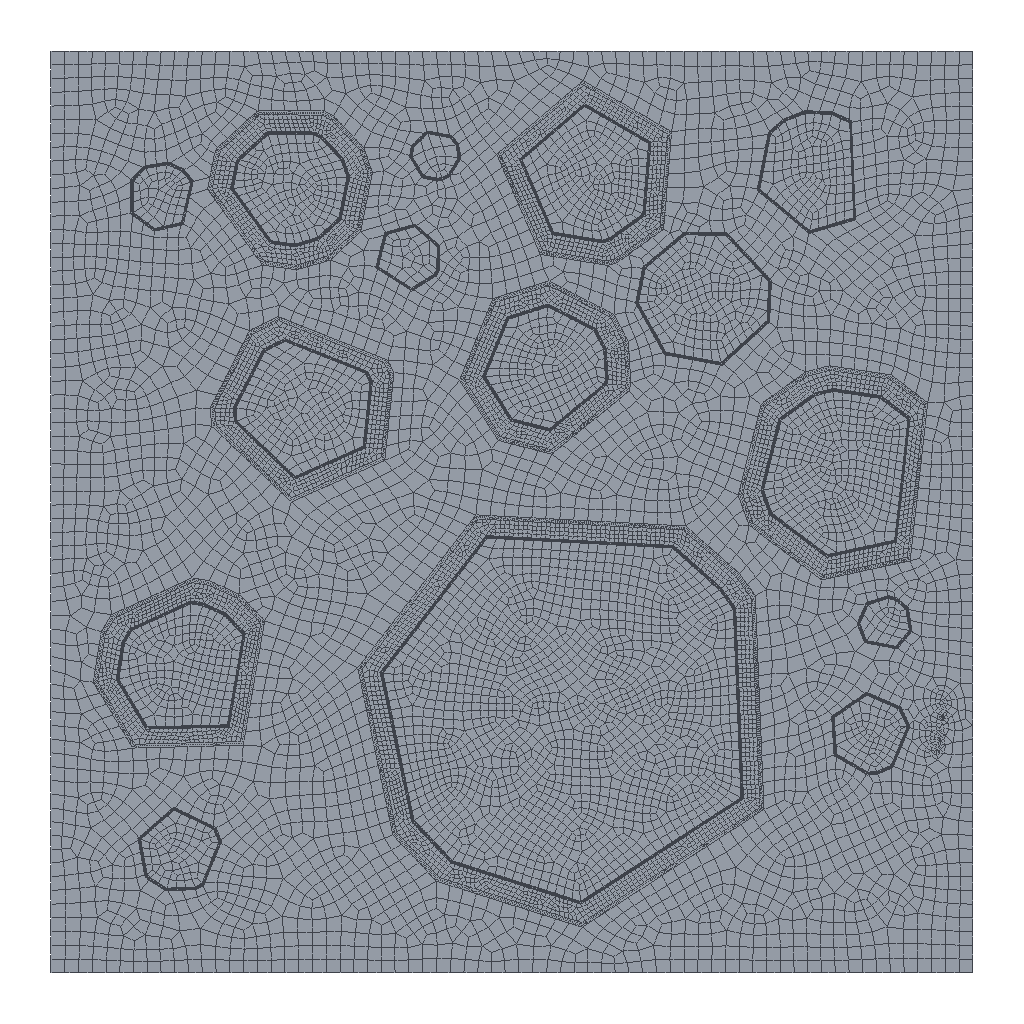Simulation study | abaqus
Set-up summary:
category,name,step,type,value,unit,region
solver,abaqus
solver,version,,,Abaqus/Standard 2020
units,not stated in the deck,,not stated
analysis,deck,,static,static
load_step,Step-1,Step-1,static
load_step,requested,,,1
mesh,nodes,,,46261
mesh,elements,,,36052
element_type,CPS4R,,plane,36052
load,load commands in deck,,count,1
bc,support commands in deck,,count,4
material,GULIAO,,in results
material,JSHANGJIANG,,in results
material,NITZ,,in results
material,NSHAJIANG,,in results
material,OITZ,,in results
check,setup vs results,,match,"per instance, exact: element labels, types and connectivity; labels of the nodes the elements use; coordinates of those nodes at SINGLE_PRECISION in 1 of 5 instance(s)"
Abaqus input file, long lists of numbers shortened:
*Heading
** Job name: Job-1 Model name: model-zaisheng
** Generated by: Abaqus/CAE 2020
*Preprint, echo=NO, model=NO, history=NO, contact=NO
**
** PARTS
**
*Part, name=Part-1
*Node
      1,   77.662,   70.73
      2,   77.846,   75.039
** (3564 more lines like these left out)
*Element, type=CPS4R
  1, 763, 677, 676, 695
  2, 715, 702, 674, 757
** (3245 more lines like these left out)
*Nset, nset=guliao-2, generate
    1,  3566,     1
*Elset, elset=guliao-2, generate
    1,  3247,     1
** Section: guliao-2
*Solid Section, elset=guliao-2, material=guliao
,
*End Part
**
*Part, name=Part-2
*Node
      1,   77.846,   75.039
      2,   77.662,   70.73
** (24805 more lines like these left out)
*Element, type=CPS4R
   1, 12276, 12405, 12781, 12812
   2, 12805, 12781, 12405, 12674
** (18677 more lines like these left out)
*Nset, nset=OITZ-2, generate
     1,  24807,      1
*Elset, elset=OITZ-2, generate
     1,  18679,      1
** Section: OITZ-2
*Solid Section, elset=OITZ-2, material=OITZ
,
*End Part
**
*Part, name=Part-3
*Node
      1,   93.19,   60.231
      2,   91.683,   46.706
** (4621 more lines like these left out)
*Element, type=CPS4R
  1,  253, 1795, 1912,  252
  2,  133, 1891, 1889,  132
** (3725 more lines like these left out)
*Nset, nset=Oshajiang-2, generate
    1,  4623,     1
*Elset, elset=Oshajiang-2, generate
    1,  3727,     1
** Section: Oshajiang-2
*Solid Section, elset=Oshajiang-2, material=Jshangjiang
,
*End Part
**
*Part, name=Part-4
*Node
      1,    94.71,   61.531
      2,   92.879,   45.103
** (9188 more lines like these left out)
*Element, type=CPS4R
  1,  529, 5118, 5141,  528
  2, 5152, 5117,  142,  143
** (6687 more lines like these left out)
*Nset, nset=NITZ, generate
    1,  9190,     1
*Elset, elset=NITZ, generate
    1,  6689,     1
** Section: NITZ-2
*Solid Section, elset=NITZ, material=NITZ
,
*End Part
**
*Part, name=Part-5
*Node
      1,   93.619,   48.661
      2,   94.207,    53.939
** (4073 more lines like these left out)
*Element, type=CPS4R
   1,  400, 2014, 2010, 2510
   2, 1384, 1385,  877,    4
** (3708 more lines like these left out)
*Nset, nset=Nshajiang-2, generate
    1,  4075,     1
*Elset, elset=Nshajiang-2, generate
    1,  3710,     1
** Section: Nshajiang-2
*Solid Section, elset=Nshajiang-2, material=Nshajiang
,
*End Part
**
**
** ASSEMBLY
**
*Assembly, name=Assembly
**
*Instance, name=Part-1-1, part=Part-1
*End Instance
**
*Instance, name=Part-2-1, part=Part-2
*End Instance
**
*Instance, name=Part-3-1, part=Part-3
*End Instance
**
*Instance, name=Part-4-1, part=Part-4
*End Instance
**
*Instance, name=Part-5-1, part=Part-5
*End Instance
**
*Node
      1,          50.,         110.,           0.
*Nset, nset=Set-20
 1,
*Nset, nset=Set-21
 1,
*Nset, nset=Set-22
 1,
*Nset, nset=Set-26
 1,
*Nset, nset=Set-31
 1,
*Nset, nset=Set-35, instance=Part-5-1
  254,  255,  256,  257,  258,  259,  260,  261,  262,  263,  264,  265,  266,  267,  268,  269
  270,  271,  272,  273,  274,  275,  276,  277,  278,  279,  280,  281,  282,  283,  284,  285
** (3 more lines like these left out)
*Elset, elset=Set-35, instance=Part-5-1
   28,   29,   31,  189,  596,  598,  608,  609,  618,  620,  628,  629,  635,  636,  637,  638
  646,  647,  648,  650,  801,  806,  809,  813,  815,  816,  817,  818,  819,  820,  821,  822
** (3 more lines like these left out)
*Nset, nset=Set-39
 1,
*Nset, nset=Set-51
 1,
*Nset, nset=Set-52
 1,
*Nset, nset=Set-RP
 1,
*Nset, nset=m_Set-28
 1,
*Nset, nset=m_Set-33
 1,
*Nset, nset=m_Set-34
 1,
*Nset, nset=m_Set-36
 1,
*Nset, nset=m_Set-37
 1,
*Nset, nset=m_Set-38, instance=Part-2-1
     1,     2,     3,     4,     5,     6,     7,     8,     9,    10,    11,    12,    13,    14,    15,    16
    17,    18,    19,    20,    21,    22,    23,    24,    25,    26,    27,    28,    29,    30,    31,    32
** (544 more lines like these left out)
*Elset, elset=m_Set-38, instance=Part-2-1, generate
    1,  6575,     1
*Nset, nset=s_Set-27
 1,
*Nset, nset=s_Set-37, instance=Part-5-1, generate
    1,  4075,     1
*Elset, elset=s_Set-37, instance=Part-5-1, generate
    1,  3710,     1
*Elset, elset=_m_Surf-2_S4, internal, instance=Part-4-1
    1,   16,   26,   50,   67,   72,   74,   85,   86,   91,   92,   96,   97,  113,  126,  130
  153,  155,  165,  201,  217,  232,  239,  255,  258,  272,  289,  301,  312,  344,  346,  348
** (37 more lines like these left out)
*Elset, elset=_m_Surf-2_S2, internal, instance=Part-4-1
    9,   10,   22,   37,   49,   51,   73,   89,   93,   94,   98,   99,  103,  111,  125,  128
  131,  132,  134,  136,  142,  144,  146,  147,  151,  152,  170,  188,  194,  197,  198,  200
** (47 more lines like these left out)
*Elset, elset=_m_Surf-2_S1, internal, instance=Part-4-1
   27,   29,   58,   62,   63,   70,   71,   76,   77,   81,   85,  107,  119,  148,  190,  266
  330,  333,  334,  336,  374,  462,  470,  565,  606,  608,  639,  640,  653,  655,  667,  777
** (33 more lines like these left out)
*Elset, elset=_m_Surf-2_S3, internal, instance=Part-4-1
   30,   31,   32,   41,   66,   68,   75,   78,   84,  105,  124,  125,  150,  178,  184,  196
  216,  262,  321,  337,  339,  342,  371,  412,  415,  440,  456,  460,  461,  472,  473,  489
** (37 more lines like these left out)
*Surface, type=ELEMENT, name=m_Surf-2
_m_Surf-2_S4, S4
_m_Surf-2_S2, S2
_m_Surf-2_S1, S1
_m_Surf-2_S3, S3
*Elset, elset=_m_Surf-7_S4, internal, instance=Part-3-1
    2,    3,    9,   10,   14,   32,   77,   79,   85,   91,   95,   98,  126,  127,  135,  150
  171,  178,  199,  201,  222,  223,  228,  229,  236,  242,  243,  248,  501,  521,  523,  526
** (14 more lines like these left out)
*Elset, elset=_m_Surf-7_S2, internal, instance=Part-3-1
    4,   66,   80,   88,  198,  200,  204,  227,  230,  234,  245,  246,  247,  250,  330,  420
  502,  503,  511,  524,  531,  533,  554,  560,  598,  601,  606,  610,  611,  642,  653,  665
** (12 more lines like these left out)
*Elset, elset=_m_Surf-7_S3, internal, instance=Part-3-1
   12,   25,   28,   40,   51,   68,   69,   70,   71,   72,   73,   78,  104,  105,  106,  112
  115,  117,  120,  134,  205,  210,  211,  213,  216,  237,  249,  318,  421,  426,  458,  460
** (10 more lines like these left out)
*Elset, elset=_m_Surf-7_S1, internal, instance=Part-3-1
   15,   22,   67,  116,  118,  119,  128,  132,  136,  137,  148,  174,  224,  225,  226,  231
  232,  233,  238,  239,  241,  251,  252,  253,  255,  256,  316,  322,  331,  333,  341,  370
** (9 more lines like these left out)
*Surface, type=ELEMENT, name=m_Surf-7
_m_Surf-7_S4, S4
_m_Surf-7_S2, S2
_m_Surf-7_S3, S3
_m_Surf-7_S1, S1
*Elset, elset=_m_Surf-9_S2, internal, instance=Part-1-1
    3,    4,    6,    8,   19,   24,   28,   31,   40,   41,   44,   45,   46,   52,   58,   70
  178,  193,  195,  211,  212,  213,  216,  221,  228,  249,  250,  255,  259,  261,  269,  271
** (10 more lines like these left out)
*Elset, elset=_m_Surf-9_S4, internal, instance=Part-1-1
    5,    7,   12,   13,   14,   15,   18,   21,   26,   29,   30,   32,   33,   42,   43,   54
   55,  188,  192,  199,  214,  215,  217,  218,  220,  235,  264,  265,  268,  272,  274,  294
** (8 more lines like these left out)
*Elset, elset=_m_Surf-9_S3, internal, instance=Part-1-1
    3,   24,   37,   62,   70,   86,  187,  191,  194,  195,  197,  198,  210,  216,  219,  227
  256,  258,  262,  280,  285,  287,  288,  290,  293,  298,  301,  302,  317,  320,  331,  333
** (6 more lines like these left out)
*Elset, elset=_m_Surf-9_S1, internal, instance=Part-1-1
    9,   13,   39,   63,  188,  201,  202,  208,  220,  226,  236,  265,  267,  268,  274,  286
  306,  315,  337,  357,  374,  377,  378,  386,  387,  402,  405,  416,  431,  468,  475,  484
** (7 more lines like these left out)
*Surface, type=ELEMENT, name=m_Surf-9
_m_Surf-9_S2, S2
_m_Surf-9_S4, S4
_m_Surf-9_S3, S3
_m_Surf-9_S1, S1
*Elset, elset=_s_Surf-2_S3, internal, instance=Part-5-1
    2,    7,    9,   20,   22,   23,   47,   50,   55,   62,   63,   65,   86,   94,   98,  102
  103,  120,  131,  154,  157,  237,  258,  260,  261,  320,  327,  328,  330,  363,  367,  369
** (6 more lines like these left out)
*Elset, elset=_s_Surf-2_S1, internal, instance=Part-5-1
    3,   19,   21,   66,  156,  160,  236,  252,  254,  255,  259,  263,  272,  350,  368,  392
  450,  456,  464,  465,  466,  469,  481,  490,  491,  497,  514,  516,  522,  574,  586,  588
** (5 more lines like these left out)
*Elset, elset=_s_Surf-2_S4, internal, instance=Part-5-1
   12,   53,   57,   72,   93,   99,  219,  235,  248,  269,  270,  271,  448,  501,  502,  570
  573,  730,  739,  742,  751,  790,  945,  973, 1059, 1084, 1176, 1223, 1224, 1227, 1296, 1299
** (1 more lines like these left out)
*Elset, elset=_s_Surf-2_S2, internal, instance=Part-5-1
   56,   74,   79,   80,  119,  217,  234,  247,  262,  276,  321,  364,  366,  411,  444,  447
  449,  451,  498,  517,  571,  580,  581,  634,  681,  683,  713,  732,  733,  740,  743,  746
** (3 more lines like these left out)
*Surface, type=ELEMENT, name=s_Surf-2
_s_Surf-2_S3, S3
_s_Surf-2_S1, S1
_s_Surf-2_S4, S4
_s_Surf-2_S2, S2
*Elset, elset=_s_Surf-4_S1, internal, instance=Part-5-1
  178,  180,  323,  325,  332,  334,  342,  343,  344,  345,  429,  472,  479,  870,  871,  874
  875,  877,  878,  880,  881,  884,  888,  892,  896,  897,  900,  903, 1776, 1789, 1837, 1838
** (1 more lines like these left out)
*Elset, elset=_s_Surf-4_S3, internal, instance=Part-5-1
  430,  473,  477,  483,  488,  489,  492,  866,  869,  918, 1451, 1454, 1457, 1462, 1463, 1470
 1471, 1843, 1844, 1932, 1934
*Elset, elset=_s_Surf-4_S4, internal, instance=Part-5-1
  868,  917, 1787
*Elset, elset=_s_Surf-4_S2, internal, instance=Part-5-1
  901,  904,  907,  908,  912, 1922
*Surface, type=ELEMENT, name=s_Surf-4
_s_Surf-4_S1, S1
_s_Surf-4_S3, S3
_s_Surf-4_S4, S4
_s_Surf-4_S2, S2
*Elset, elset=_s_Surf-5_S1, internal, instance=Part-5-1
  178,  180,  323,  325,  332,  334,  342,  343,  344,  345,  429,  472,  479,  870,  871,  874
  875,  877,  878,  880,  881,  884,  888,  892,  896,  897,  900,  903, 1776, 1789, 1837, 1838
** (1 more lines like these left out)
*Elset, elset=_s_Surf-5_S3, internal, instance=Part-5-1
  430,  473,  477,  483,  488,  489,  492,  866,  869,  918, 1451, 1454, 1457, 1462, 1463, 1470
 1471, 1843, 1844, 1932, 1934
*Elset, elset=_s_Surf-5_S4, internal, instance=Part-5-1
  868,  917, 1787
*Elset, elset=_s_Surf-5_S2, internal, instance=Part-5-1
  901,  904,  907,  908,  912, 1922
*Surface, type=ELEMENT, name=s_Surf-5
_s_Surf-5_S1, S1
_s_Surf-5_S3, S3
_s_Surf-5_S4, S4
_s_Surf-5_S2, S2
*Elset, elset=_s_Surf-6_S4, internal, instance=Part-3-1
    1,   45,   57,   63,   65,   90,   93,   97,  139,  141,  144,  151,  152,  158,  162,  167
  173,  182,  187,  195,  218,  221,  265,  268,  272,  278,  279,  286,  289,  292,  294,  297
** (16 more lines like these left out)
*Elset, elset=_s_Surf-6_S2, internal, instance=Part-3-1
    7,   47,   59,   60,   82,   83,   87,   99,  100,  101,  102,  107,  108,  109,  121,  124
  143,  146,  149,  157,  159,  161,  168,  170,  172,  179,  185,  197,  206,  262,  263,  264
** (18 more lines like these left out)
*Elset, elset=_s_Surf-6_S1, internal, instance=Part-3-1
   13,   24,   27,   31,   34,   36,   42,   49,  110,  131,  141,  152,  164,  188,  257,  274
  281,  290,  313,  349,  390,  391,  505,  509,  517,  518,  525,  530,  564,  569,  570,  584
** (11 more lines like these left out)
*Elset, elset=_s_Surf-6_S3, internal, instance=Part-3-1
   16,   20,   30,   76,  155,  176,  184,  191,  193,  209,  258,  259,  260,  266,  275,  291
  339,  344,  345,  388,  506,  508,  515,  516,  529,  532,  565,  571,  572,  586,  623,  629
** (11 more lines like these left out)
*Surface, type=ELEMENT, name=s_Surf-6
_s_Surf-6_S4, S4
_s_Surf-6_S2, S2
_s_Surf-6_S1, S1
_s_Surf-6_S3, S3
*Elset, elset=_s_Surf-7_S4, internal, instance=Part-2-1
  6579,  6585,  6587,  6588,  6591,  6597,  6598,  6600,  6601,  6606,  6614,  6616,  6620,  6621,  6623,  6625
  6626,  6627,  6628,  6629,  6633,  6637,  6644,  6648,  6649,  6655,  6656,  6658,  6659,  6668,  6669,  6671
** (59 more lines like these left out)
*Elset, elset=_s_Surf-7_S2, internal, instance=Part-2-1
  6583,  6589,  6604,  6605,  6610,  6612,  6618,  6632,  6636,  6639,  6641,  6642,  6650,  6651,  6652,  6673
  6676,  6679,  6680,  6682,  6683,  6688,  6689,  6690,  6699,  6703,  6710,  6784,  6813,  6815,  6823,  6830
** (72 more lines like these left out)
*Elset, elset=_s_Surf-7_S1, internal, instance=Part-2-1
  6691,  6711,  6719,  6727,  6749,  6759,  6760,  6761,  6785,  6806,  6814,  6819,  6822,  6825,  6827,  6831
  6837,  6841,  6851,  6878,  6929,  6930,  6934,  6935,  6997,  7008,  7020,  7060,  7147,  7223,  7243,  7246
** (62 more lines like these left out)
*Elset, elset=_s_Surf-7_S3, internal, instance=Part-2-1
  6715,  6756,  6763,  6767,  6773,  6786,  6790,  6791,  6794,  6797,  6836,  6838,  6840,  6843,  6849,  6854
  6882,  6928,  6983,  6985,  6992,  6993,  6995,  7009,  7017,  7085,  7114,  7149,  7158,  7206,  7217,  7220
** (54 more lines like these left out)
*Surface, type=ELEMENT, name=s_Surf-7
_s_Surf-7_S4, S4
_s_Surf-7_S2, S2
_s_Surf-7_S1, S1
_s_Surf-7_S3, S3
*Elset, elset=_s_Surf-9_S3, internal, instance=Part-2-1
     5,     6,     7,    11,    21,    37,    41,    60,    68,    71,    82,   227,   228,   230,   238,   242
   254,   259,   262,   266,   268,   281,   293,   298,   300,   302,   303,   304,   329,   331,   332,   344
** (94 more lines like these left out)
*Elset, elset=_s_Surf-9_S1, internal, instance=Part-2-1
    12,    18,    19,    22,    27,    29,    31,    39,    47,    48,    57,    59,    64,    65,    67,    75
    78,    80,   120,   235,   239,   246,   269,   271,   276,   280,   289,   290,   296,   299,   308,   327
** (98 more lines like these left out)
*Elset, elset=_s_Surf-9_S2, internal, instance=Part-2-1
    88,    97,   106,   107,   131,   133,   142,   146,   149,   150,   155,   174,   176,   194,   213,   245
   307,   319,   333,   336,   354,   357,   366,   376,   377,   378,   628,   646,   669,   711,   712,   713
** (97 more lines like these left out)
*Elset, elset=_s_Surf-9_S4, internal, instance=Part-2-1
    84,    94,   102,   112,   116,   139,   140,   148,   152,   153,   154,   163,   165,   169,   178,   179
   182,   189,   190,   199,   214,   219,   222,   223,   240,   317,   322,   335,   352,   363,   554,   610
** (80 more lines like these left out)
*Surface, type=ELEMENT, name=s_Surf-9
_s_Surf-9_S3, S3
_s_Surf-9_S1, S1
_s_Surf-9_S2, S2
_s_Surf-9_S4, S4
** Constraint: Constraint-1
*Tie, name=Constraint-1, adjust=yes
m_Surf-2, s_Surf-2
** Constraint: Constraint-2
*Coupling, constraint name=Constraint-2, ref node=m_Set-36, surface=s_Surf-5
*Kinematic
** Constraint: Constraint-3
*Tie, name=Constraint-3, adjust=yes
s_Surf-6, m_Surf-2
** Constraint: Constraint-guliao
*Tie, name=Constraint-guliao, adjust=yes
m_Surf-9, s_Surf-9
** Constraint: Constraint-insert
*Embedded Element, host elset=s_Set-37
m_Set-38
** Constraint: Constraint-p2-p3
*Tie, name=Constraint-p2-p3, adjust=yes
s_Surf-7, m_Surf-7
*End Assembly
*Amplitude, name=Amp-2, definition=SMOOTH STEP
             0.,              0.,           0.001,              1.
*Amplitude, name=Amp-3
             0.,              0.,              1.,              1.
*Amplitude, name=Amp-4, definition=SMOOTH STEP
             0.,              0.,           0.001,              1.
**
** MATERIALS
**
*Material, name=Jshangjiang
*Density
 2.36e-09,
*Elastic
 20396.2, 0.22
*Concrete Damaged Plasticity
36.,    0.1,   1.16,  0.667, 0.0005
*Concrete Compression Hardening
 17.812,          0.
 19.451, 3.76892e-05
 20.955,  7.4105e-05
 22.323, 0.0001172
 23.552, 0.0001671
 24.642, 0.0002238
 25.591, 0.0002874
 26.398,  0.000358
 24.688, 0.000552
 26.246, 0.0005858
 27.373, 0.0006406
  28.038,   0.0007182
  28.251,  0.0008179
 28.058, 0.0009375
 27.529,  0.001074
  26.741,  0.001222
 25.772,  0.00138
 24.688,  0.001543
 23.546,  0.001709
  22.388,  0.001876
 21.244,  0.002043
 20.136,  0.002207
 19.076,  0.002369
 18.072,  0.002529
 17.129,  0.002685
 16.246,  0.002838
 15.422,  0.002989
 14.656,  0.003137
 13.943,  0.003282
 13.281,  0.003424
 12.667,  0.003565
 12.095,  0.003703
 11.564,  0.003839
 9.779,   0.004367
*Concrete Tension Stiffening
 2.06,      0.
 1.92,   2e-05
 1.72,   5e-05
 1.53,   8e-05
 1.37,  0.0001
 1.24, 0.00013
 1.13, 0.00015
 1.04, 0.00017
 0.97, 0.00019
  0.9, 0.00021
 0.85, 0.00024
 0.66, 0.00033
 0.54, 0.00043
 0.47, 0.00052
 0.41, 0.00062
 0.37, 0.00071
 0.34,  0.0008
 0.31, 0.00089
 0.29, 0.00099
*Concrete Compression Damage, tension recovery=1.
        0.,          0.
 0.01172, 3.76892e-05
 0.02118,  7.4105e-05
 0.03113, 0.0001172
  0.04161, 0.0001671
 0.05265, 0.0002238
 0.0643, 0.0002874
 0.07663,  0.000358
   0.1203, 0.000552
  0.1202, 0.0005858
  0.1253, 0.0006406
  0.1355,   0.0007182
  0.1505,  0.0008179
  0.1697, 0.0009375
  0.1927,  0.001074
  0.2186,  0.001222
  0.2468,  0.00138
  0.2767,  0.001543
   0.3076,  0.001709
  0.339,  0.001876
  0.3704,  0.002043
  0.4015,  0.002207
  0.4318,  0.002369
  0.4612,  0.002529
  0.4896,  0.002685
  0.5167,  0.002838
  0.5425,  0.002989
  0.567,  0.003137
  0.5902,  0.003282
   0.612,  0.003424
  0.6326,  0.003565
  0.652,  0.003703
  0.6701,  0.003839
  0.7321,   0.004367
*Concrete Tension Damage
      0.,      0.
 0.1393,   2e-05
 0.2776,   5e-05
 0.3954,   8e-05
 0.4912,  0.0001
 0.5681, 0.00013
 0.6297, 0.00015
 0.6794, 0.00017
 0.7199, 0.00019
 0.7533, 0.00021
 0.781, 0.00024
 0.8675, 0.00033
 0.9105, 0.00043
 0.935, 0.00052
 0.9504, 0.00062
 0.9607, 0.00071
 0.9679,  0.0008
 0.9733, 0.00089
 0.9774, 0.00099
*Material, name=NITZ
*Density
 2.37e-09,
*Elastic
 19263.1, 0.2
*Concrete Damaged Plasticity
30.,    0.1,   1.16,  0.667, 0.0005
*Concrete Compression Hardening
 16.823,          0.
 18.371, 3.76892e-05
  19.791,  7.4105e-05
 21.082, 0.0001172
 22.243, 0.0001671
 23.273, 0.0002238
 24.169, 0.0002874
 24.931,  0.000358
 23.317, 0.000552
 24.788, 0.0005858
 25.852, 0.0006406
 26.48,   0.0007182
 26.681,  0.0008179
 26.499, 0.0009375
 25.999,  0.001074
 25.255,  0.001222
   24.34,  0.00138
 23.317,  0.001543
 22.238,  0.001709
 21.144,  0.001876
 20.064,  0.002043
 19.017,  0.002207
 18.016,  0.002369
 17.068,  0.002529
  16.177,  0.002685
 15.343,  0.002838
 14.565,  0.002989
 13.841,  0.003137
 13.169,  0.003282
 12.544,  0.003424
 11.963,  0.003565
 11.423,  0.003703
 10.922,  0.003839
 9.235,   0.004367
*Concrete Tension Stiffening
 2.06,      0.
 1.92,   2e-05
 1.72,   5e-05
 1.53,   8e-05
 1.37,  0.0001
 1.24, 0.00013
 1.13, 0.00015
 1.04, 0.00017
 0.97, 0.00019
  0.9, 0.00021
 0.85, 0.00024
 0.66, 0.00033
 0.54, 0.00043
 0.47, 0.00052
 0.41, 0.00062
 0.37, 0.00071
 0.34,  0.0008
 0.31, 0.00089
 0.29, 0.00099
*Concrete Compression Damage
        0.,          0.
 0.01172, 3.76892e-05
 0.02118,  7.4105e-05
 0.03113, 0.0001172
  0.04161, 0.0001671
 0.05265, 0.0002238
 0.0643, 0.0002874
 0.07663,  0.000358
   0.1203, 0.000552
  0.1202, 0.0005858
  0.1253, 0.0006406
  0.1355,   0.0007182
  0.1505,  0.0008179
  0.1697, 0.0009375
  0.1927,  0.001074
  0.2186,  0.001222
  0.2468,  0.00138
  0.2767,  0.001543
   0.3076,  0.001709
  0.339,  0.001876
  0.3704,  0.002043
  0.4015,  0.002207
  0.4318,  0.002369
  0.4612,  0.002529
  0.4896,  0.002685
  0.5167,  0.002838
  0.5425,  0.002989
  0.567,  0.003137
  0.5902,  0.003282
   0.612,  0.003424
  0.6326,  0.003565
  0.652,  0.003703
  0.6701,  0.003839
  0.7321,   0.004367
*Concrete Tension Damage
      0.,      0.
 0.1393,   2e-05
 0.2776,   5e-05
 0.3954,   8e-05
 0.4912,  0.0001
 0.5681, 0.00013
 0.6297, 0.00015
 0.6794, 0.00017
 0.7199, 0.00019
 0.7533, 0.00021
 0.781, 0.00024
 0.8675, 0.00033
 0.9105, 0.00043
 0.935, 0.00052
 0.9504, 0.00062
 0.9607, 0.00071
 0.9679,  0.0008
 0.9733, 0.00089
 0.9774, 0.00099
*Material, name=Nshajiang
*Density
 2.38e-09,
*Elastic
 22662.5, 0.22
*Concrete Damaged Plasticity
36.,    0.1,   1.16,  0.667, 0.0005
*Concrete Compression Hardening
 15.14,          0.
 16.534, 3.76892e-05
 17.812,  7.4105e-05
 18.974, 0.0001172
 20.019, 0.0001671
 20.945, 0.0002238
 21.752, 0.0002874
 22.438,  0.000358
 20.985, 0.000552
 22.309, 0.0005858
 23.267, 0.0006406
 23.832,   0.0007182
 24.013,  0.0008179
 23.849, 0.0009375
 23.399,  0.001074
 22.73,  0.001222
  21.906,  0.00138
 20.985,  0.001543
 20.014,  0.001709
 19.03,  0.001876
 18.058,  0.002043
 17.115,  0.002207
 16.214,  0.002369
 15.361,  0.002529
 14.559,  0.002685
 13.809,  0.002838
 13.109,  0.002989
 12.457,  0.003137
 11.852,  0.003282
 11.289,  0.003424
 10.767,  0.003565
  10.281,  0.003703
 9.829,  0.003839
 8.312,   0.004367
*Concrete Tension Stiffening
 2.06,      0.
 1.92,   2e-05
 1.72,   5e-05
 1.53,   8e-05
 1.37,  0.0001
 1.24, 0.00013
 1.13, 0.00015
 1.04, 0.00017
 0.97, 0.00019
  0.9, 0.00021
 0.85, 0.00024
 0.66, 0.00033
 0.54, 0.00043
 0.47, 0.00052
 0.41, 0.00062
 0.37, 0.00071
 0.34,  0.0008
 0.31, 0.00089
 0.29, 0.00099
*Concrete Compression Damage, tension recovery=1.
        0.,          0.
 0.01172, 3.76892e-05
 0.02118,  7.4105e-05
 0.03113, 0.0001172
  0.04161, 0.0001671
 0.05265, 0.0002238
 0.0643, 0.0002874
 0.07663,  0.000358
   0.1203, 0.000552
  0.1202, 0.0005858
  0.1253, 0.0006406
  0.1355,   0.0007182
  0.1505,  0.0008179
  0.1697, 0.0009375
  0.1927,  0.001074
  0.2186,  0.001222
  0.2468,  0.00138
  0.2767,  0.001543
   0.3076,  0.001709
  0.339,  0.001876
  0.3704,  0.002043
  0.4015,  0.002207
  0.4318,  0.002369
  0.4612,  0.002529
  0.4896,  0.002685
  0.5167,  0.002838
  0.5425,  0.002989
  0.567,  0.003137
  0.5902,  0.003282
   0.612,  0.003424
  0.6326,  0.003565
  0.652,  0.003703
  0.6701,  0.003839
  0.7321,   0.004367
*Concrete Tension Damage
      0.,      0.
 0.1393,   2e-05
 0.2776,   5e-05
 0.3954,   8e-05
 0.4912,  0.0001
 0.5681, 0.00013
 0.6297, 0.00015
 0.6794, 0.00017
 0.7199, 0.00019
 0.7533, 0.00021
 0.781, 0.00024
 0.8675, 0.00033
 0.9105, 0.00043
 0.935, 0.00052
 0.9504, 0.00062
 0.9607, 0.00071
 0.9679,  0.0008
 0.9733, 0.00089
 0.9774, 0.00099
*Material, name=OITZ
*Density
 2.37e-09,
*Elastic
 17336.8, 0.2
*Concrete Damaged Plasticity
30.,    0.1,   1.16,  0.667, 0.0005
*Concrete Compression Hardening
 19.791,          0.
 21.613, 3.76892e-05
 23.284,  7.4105e-05
 24.803, 0.0001172
 26.169, 0.0001671
 27.38, 0.0002238
 28.434, 0.0002874
  29.331,  0.000358
 27.432, 0.000552
 29.162, 0.0005858
 30.415, 0.0006406
 31.153,   0.0007182
   31.39,  0.0008179
 31.176, 0.0009375
 30.587,  0.001074
 29.712,  0.001222
 28.635,  0.00138
 27.432,  0.001543
 26.163,  0.001709
 24.876,  0.001876
 23.605,  0.002043
 22.373,  0.002207
 21.195,  0.002369
 20.08,  0.002529
 19.032,  0.002685
 18.051,  0.002838
 17.136,  0.002989
 16.284,  0.003137
 15.493,  0.003282
 14.757,  0.003424
  14.074,  0.003565
 13.439,  0.003703
 12.849,  0.003839
 10.865,   0.004367
*Concrete Tension Stiffening
 2.06,      0.
 1.92,   2e-05
 1.72,   5e-05
 1.53,   8e-05
 1.37,  0.0001
 1.24, 0.00013
 1.13, 0.00015
 1.04, 0.00017
 0.97, 0.00019
  0.9, 0.00021
 0.85, 0.00024
 0.66, 0.00033
 0.54, 0.00043
 0.47, 0.00052
 0.41, 0.00062
 0.37, 0.00071
 0.34,  0.0008
 0.31, 0.00089
 0.29, 0.00099
*Concrete Compression Damage, tension recovery=1.
        0.,          0.
 0.01172, 3.76892e-05
 0.02118,  7.4105e-05
 0.03113, 0.0001172
  0.04161, 0.0001671
 0.05265, 0.0002238
 0.0643, 0.0002874
 0.07663,  0.000358
   0.1203, 0.000552
  0.1202, 0.0005858
  0.1253, 0.0006406
  0.1355,   0.0007182
  0.1505,  0.0008179
  0.1697, 0.0009375
  0.1927,  0.001074
  0.2186,  0.001222
  0.2468,  0.00138
  0.2767,  0.001543
   0.3076,  0.001709
  0.339,  0.001876
  0.3704,  0.002043
  0.4015,  0.002207
  0.4318,  0.002369
  0.4612,  0.002529
  0.4896,  0.002685
  0.5167,  0.002838
  0.5425,  0.002989
  0.567,  0.003137
  0.5902,  0.003282
   0.612,  0.003424
  0.6326,  0.003565
  0.652,  0.003703
  0.6701,  0.003839
  0.7321,   0.004367
*Concrete Tension Damage
      0.,      0.
 0.1393,   2e-05
 0.2776,   5e-05
 0.3954,   8e-05
 0.4912,  0.0001
 0.5681, 0.00013
 0.6297, 0.00015
 0.6794, 0.00017
 0.7199, 0.00019
 0.7533, 0.00021
 0.781, 0.00024
 0.8675, 0.00033
 0.9105, 0.00043
 0.935, 0.00052
 0.9504, 0.00062
 0.9607, 0.00071
 0.9679,  0.0008
 0.9733, 0.00089
 0.9774, 0.00099
*Material, name=guliao
*Density
 2.37e-09,
*Elastic
70000., 0.16
**
** INTERACTION PROPERTIES
**
*Surface Interaction, name=IntProp-1
1.,
*Friction
0.,
*Surface Behavior, pressure-overclosure=HARD
** ----------------------------------------------------------------
**
** STEP: Step-1
**
*Step, name=Step-1, nlgeom=YES, inc=10000
*Static, stabilize=0.0002, allsdtol=0.05, continue=NO
0.001, 1., 1e-09, 1.
**
** BOUNDARY CONDITIONS
**
** Name: BC-2 Type: 位移/转角
*Boundary, amplitude=Amp-4
Set-RP, 1, 1
Set-RP, 2, 2, -0.5
Set-RP, 6, 6
** Name: BC-3 Type: 对称/反对称/完全固定
*Boundary
Set-35, ENCASTRE
**
** OUTPUT REQUESTS
**
*Restart, write, frequency=0
**
** FIELD OUTPUT: F-Output-1
**
*Output, field
*Node Output
RF, RT, U, V
*Element Output, directions=YES
DAMAGEC, DAMAGET, DMICRT, E, LE, MISES, MISESMAX, PE, PEEQ, PEMAG, S, SDEG, STATUS
*Contact Output
CDISP, CSTRESS
**
** HISTORY OUTPUT: H-Output-1
**
*Output, history
*Node Output, nset=m_Set-36
RF2, U2
*End Step
Results summary:
result,step,,partial,increments=13 time=0.0001277/1.0
result,analysis,,,static
result,last_loadstep,,,1
result,primary field,,,U
result,reaction total,,FX,0.1189,model units
result,reaction total,,FY,-2.817,model units
result,reaction total,,FZ,0.0,model units